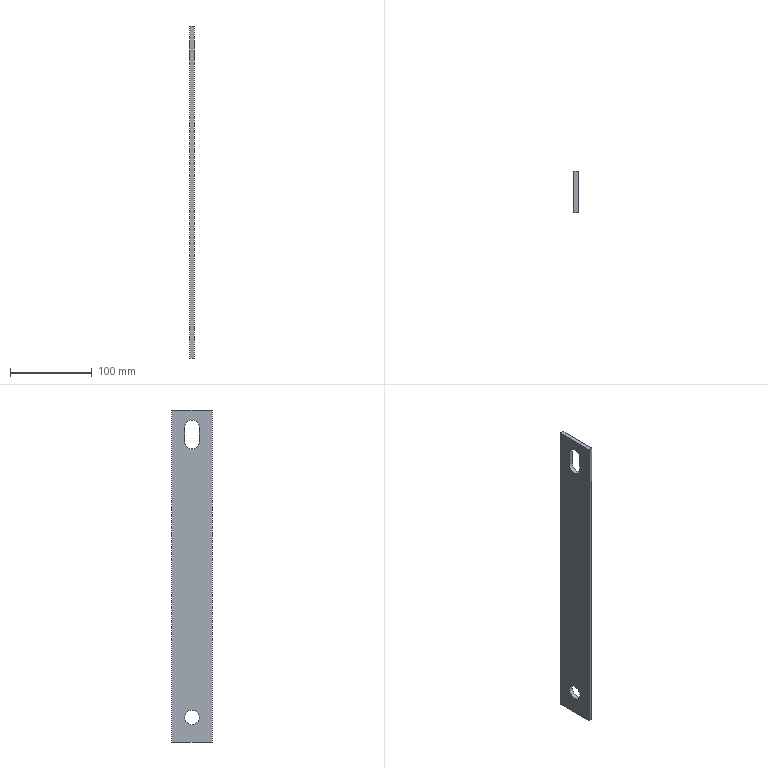Part | NX | features solid 2 | 1 solid | 11 faces | box 5 x 50 x 405 mm | volume 97175 mm3 | plane 8 | cylinder 3 | commonest cylinder face diameters 18 x3
STEP:
#1=CARTESIAN_POINT('',(1280.,720.,-185.));
#2=VERTEX_POINT('',#1);
#3=CARTESIAN_POINT('',(1280.,670.,-185.));
#4=VERTEX_POINT('',#3);
#5=CARTESIAN_POINT('',(1280.,695.,-185.));
#6=DIRECTION('',(0.,-1.,0.));
#7=VECTOR('',#6,1000.);
#8=LINE('',#5,#7);
#9=EDGE_CURVE('',#2,#4,#8,.T.);
#10=ORIENTED_EDGE('',*,*,#9,.F.);
#11=CARTESIAN_POINT('',(1285.,720.,-185.));
#12=VERTEX_POINT('',#11);
#13=CARTESIAN_POINT('',(1282.5,720.,-185.));
#14=DIRECTION('',(-1.,0.,0.));
#15=VECTOR('',#14,1000.);
#16=LINE('',#13,#15);
#17=EDGE_CURVE('',#12,#2,#16,.T.);
#18=ORIENTED_EDGE('',*,*,#17,.F.);
#19=CARTESIAN_POINT('',(1285.,670.,-185.));
#20=VERTEX_POINT('',#19);
#21=CARTESIAN_POINT('',(1285.,695.,-185.));
#22=DIRECTION('',(0.,1.,0.));
#23=VECTOR('',#22,1000.);
#24=LINE('',#21,#23);
#25=EDGE_CURVE('',#20,#12,#24,.T.);
#26=ORIENTED_EDGE('',*,*,#25,.F.);
#27=CARTESIAN_POINT('',(1282.5,670.,-185.));
#28=DIRECTION('',(1.,0.,0.));
#29=VECTOR('',#28,1000.);
#30=LINE('',#27,#29);
#31=EDGE_CURVE('',#4,#20,#30,.T.);
#32=ORIENTED_EDGE('',*,*,#31,.F.);
#33=EDGE_LOOP('',(#10,#18,#26,#32));
#34=FACE_BOUND('',#33,.T.);
#35=CARTESIAN_POINT('',(1272.5,695.,-185.));
#36=DIRECTION('',(0.,0.,-1.));
#37=DIRECTION('',(1.,0.,0.));
#38=AXIS2_PLACEMENT_3D('',#35,#36,#37);
#39=PLANE('',#38);
#40=ADVANCED_FACE('',(#34),#39,.T.);
#41=CARTESIAN_POINT('',(1285.,695.,-164.));
#42=VERTEX_POINT('',#41);
#43=CARTESIAN_POINT('',(1285.,695.,-155.));
#44=DIRECTION('',(-1.,0.,0.));
#45=DIRECTION('',(0.,0.,-1.));
#46=AXIS2_PLACEMENT_3D('',#43,#44,#45);
#47=CIRCLE('',#46,9.);
#48=EDGE_CURVE('',#42,#42,#47,.T.);
#49=ORIENTED_EDGE('',*,*,#48,.F.);
#50=EDGE_LOOP('',(#49));
#51=FACE_BOUND('',#50,.T.);
#52=CARTESIAN_POINT('',(1280.,695.,-146.));
#53=VERTEX_POINT('',#52);
#54=CARTESIAN_POINT('',(1280.,695.,-155.));
#55=DIRECTION('',(1.,0.,0.));
#56=DIRECTION('',(0.,0.,1.));
#57=AXIS2_PLACEMENT_3D('',#54,#55,#56);
#58=CIRCLE('',#57,9.);
#59=EDGE_CURVE('',#53,#53,#58,.T.);
#60=ORIENTED_EDGE('',*,*,#59,.F.);
#61=EDGE_LOOP('',(#60));
#62=FACE_BOUND('',#61,.T.);
#63=CARTESIAN_POINT('',(1280.,695.,-155.));
#64=DIRECTION('',(1.,0.,0.));
#65=DIRECTION('',(0.,0.,1.));
#66=AXIS2_PLACEMENT_3D('',#63,#64,#65);
#67=CYLINDRICAL_SURFACE('',#66,9.);
#68=ADVANCED_FACE('',(#51,#62),#67,.F.);
#69=ORIENTED_EDGE('',*,*,#59,.T.);
#70=EDGE_LOOP('',(#69));
#71=FACE_BOUND('',#70,.T.);
#72=CARTESIAN_POINT('',(1280.,670.,220.));
#73=VERTEX_POINT('',#72);
#74=CARTESIAN_POINT('',(1280.,670.,-215.));
#75=DIRECTION('',(0.,0.,1.));
#76=VECTOR('',#75,1000.);
#77=LINE('',#74,#76);
#78=EDGE_CURVE('',#4,#73,#77,.T.);
#79=ORIENTED_EDGE('',*,*,#78,.T.);
#80=CARTESIAN_POINT('',(1280.,720.,220.));
#81=VERTEX_POINT('',#80);
#82=CARTESIAN_POINT('',(1280.,695.,220.));
#83=DIRECTION('',(0.,1.,0.));
#84=VECTOR('',#83,1000.);
#85=LINE('',#82,#84);
#86=EDGE_CURVE('',#73,#81,#85,.T.);
#87=ORIENTED_EDGE('',*,*,#86,.T.);
#88=CARTESIAN_POINT('',(1280.,720.,-215.));
#89=DIRECTION('',(0.,0.,1.));
#90=VECTOR('',#89,1000.);
#91=LINE('',#88,#90);
#92=EDGE_CURVE('',#2,#81,#91,.T.);
#93=ORIENTED_EDGE('',*,*,#92,.F.);
#94=ORIENTED_EDGE('',*,*,#9,.T.);
#95=EDGE_LOOP('',(#79,#87,#93,#94));
#96=FACE_BOUND('',#95,.T.);
#97=CARTESIAN_POINT('',(1280.,704.,181.5));
#98=VERTEX_POINT('',#97);
#99=CARTESIAN_POINT('',(1280.,704.,198.5));
#100=VERTEX_POINT('',#99);
#101=CARTESIAN_POINT('',(1280.,704.,181.5));
#102=DIRECTION('',(0.,0.,1.));
#103=VECTOR('',#102,1000.);
#104=LINE('',#101,#103);
#105=EDGE_CURVE('',#98,#100,#104,.T.);
#106=ORIENTED_EDGE('',*,*,#105,.T.);
#107=CARTESIAN_POINT('',(1280.,686.,198.5));
#108=VERTEX_POINT('',#107);
#109=CARTESIAN_POINT('',(1280.,695.,198.5));
#110=DIRECTION('',(1.,0.,0.));
#111=DIRECTION('',(0.,0.,1.));
#112=AXIS2_PLACEMENT_3D('',#109,#110,#111);
#113=CIRCLE('',#112,9.);
#114=EDGE_CURVE('',#100,#108,#113,.T.);
#115=ORIENTED_EDGE('',*,*,#114,.T.);
#116=CARTESIAN_POINT('',(1280.,686.,181.5));
#117=VERTEX_POINT('',#116);
#118=CARTESIAN_POINT('',(1280.,686.,181.5));
#119=DIRECTION('',(0.,0.,1.));
#120=VECTOR('',#119,1000.);
#121=LINE('',#118,#120);
#122=EDGE_CURVE('',#117,#108,#121,.T.);
#123=ORIENTED_EDGE('',*,*,#122,.F.);
#124=CARTESIAN_POINT('',(1280.,695.,181.5));
#125=DIRECTION('',(1.,0.,0.));
#126=DIRECTION('',(0.,0.,1.));
#127=AXIS2_PLACEMENT_3D('',#124,#125,#126);
#128=CIRCLE('',#127,9.);
#129=EDGE_CURVE('',#117,#98,#128,.T.);
#130=ORIENTED_EDGE('',*,*,#129,.T.);
#131=EDGE_LOOP('',(#106,#115,#123,#130));
#132=FACE_BOUND('',#131,.T.);
#133=CARTESIAN_POINT('',(1280.,695.,-215.));
#134=DIRECTION('',(-1.,0.,0.));
#135=DIRECTION('',(0.,0.,-1.));
#136=AXIS2_PLACEMENT_3D('',#133,#134,#135);
#137=PLANE('',#136);
#138=ADVANCED_FACE('',(#71,#96,#132),#137,.T.);
#139=CARTESIAN_POINT('',(1285.,670.,220.));
#140=VERTEX_POINT('',#139);
#141=CARTESIAN_POINT('',(1285.,670.,-215.));
#142=DIRECTION('',(0.,0.,1.));
#143=VECTOR('',#142,1000.);
#144=LINE('',#141,#143);
#145=EDGE_CURVE('',#20,#140,#144,.T.);
#146=ORIENTED_EDGE('',*,*,#145,.T.);
#147=CARTESIAN_POINT('',(1282.5,670.,220.));
#148=DIRECTION('',(-1.,0.,0.));
#149=VECTOR('',#148,1000.);
#150=LINE('',#147,#149);
#151=EDGE_CURVE('',#140,#73,#150,.T.);
#152=ORIENTED_EDGE('',*,*,#151,.T.);
#153=ORIENTED_EDGE('',*,*,#78,.F.);
#154=ORIENTED_EDGE('',*,*,#31,.T.);
#155=EDGE_LOOP('',(#146,#152,#153,#154));
#156=FACE_BOUND('',#155,.T.);
#157=CARTESIAN_POINT('',(1282.5,670.,-215.));
#158=DIRECTION('',(0.,-1.,0.));
#159=DIRECTION('',(0.,0.,1.));
#160=AXIS2_PLACEMENT_3D('',#157,#158,#159);
#161=PLANE('',#160);
#162=ADVANCED_FACE('',(#156),#161,.T.);
#163=ORIENTED_EDGE('',*,*,#48,.T.);
#164=EDGE_LOOP('',(#163));
#165=FACE_BOUND('',#164,.T.);
#166=CARTESIAN_POINT('',(1285.,720.,220.));
#167=VERTEX_POINT('',#166);
#168=CARTESIAN_POINT('',(1285.,720.,-215.));
#169=DIRECTION('',(0.,0.,1.));
#170=VECTOR('',#169,1000.);
#171=LINE('',#168,#170);
#172=EDGE_CURVE('',#12,#167,#171,.T.);
#173=ORIENTED_EDGE('',*,*,#172,.T.);
#174=CARTESIAN_POINT('',(1285.,695.,220.));
#175=DIRECTION('',(0.,-1.,0.));
#176=VECTOR('',#175,1000.);
#177=LINE('',#174,#176);
#178=EDGE_CURVE('',#167,#140,#177,.T.);
#179=ORIENTED_EDGE('',*,*,#178,.T.);
#180=ORIENTED_EDGE('',*,*,#145,.F.);
#181=ORIENTED_EDGE('',*,*,#25,.T.);
#182=EDGE_LOOP('',(#173,#179,#180,#181));
#183=FACE_BOUND('',#182,.T.);
#184=CARTESIAN_POINT('',(1285.,704.,181.5));
#185=VERTEX_POINT('',#184);
#186=CARTESIAN_POINT('',(1285.,704.,198.5));
#187=VERTEX_POINT('',#186);
#188=CARTESIAN_POINT('',(1285.,704.,181.5));
#189=DIRECTION('',(0.,0.,1.));
#190=VECTOR('',#189,1000.);
#191=LINE('',#188,#190);
#192=EDGE_CURVE('',#185,#187,#191,.T.);
#193=ORIENTED_EDGE('',*,*,#192,.F.);
#194=CARTESIAN_POINT('',(1285.,686.,181.5));
#195=VERTEX_POINT('',#194);
#196=CARTESIAN_POINT('',(1285.,695.,181.5));
#197=DIRECTION('',(-1.,0.,0.));
#198=DIRECTION('',(0.,0.,-1.));
#199=AXIS2_PLACEMENT_3D('',#196,#197,#198);
#200=CIRCLE('',#199,9.);
#201=EDGE_CURVE('',#185,#195,#200,.T.);
#202=ORIENTED_EDGE('',*,*,#201,.T.);
#203=CARTESIAN_POINT('',(1285.,686.,198.5));
#204=VERTEX_POINT('',#203);
#205=CARTESIAN_POINT('',(1285.,686.,181.5));
#206=DIRECTION('',(0.,0.,1.));
#207=VECTOR('',#206,1000.);
#208=LINE('',#205,#207);
#209=EDGE_CURVE('',#195,#204,#208,.T.);
#210=ORIENTED_EDGE('',*,*,#209,.T.);
#211=CARTESIAN_POINT('',(1285.,695.,198.5));
#212=DIRECTION('',(-1.,0.,0.));
#213=DIRECTION('',(0.,0.,-1.));
#214=AXIS2_PLACEMENT_3D('',#211,#212,#213);
#215=CIRCLE('',#214,9.);
#216=EDGE_CURVE('',#204,#187,#215,.T.);
#217=ORIENTED_EDGE('',*,*,#216,.T.);
#218=EDGE_LOOP('',(#193,#202,#210,#217));
#219=FACE_BOUND('',#218,.T.);
#220=CARTESIAN_POINT('',(1285.,695.,-215.));
#221=DIRECTION('',(1.,0.,0.));
#222=DIRECTION('',(0.,0.,1.));
#223=AXIS2_PLACEMENT_3D('',#220,#221,#222);
#224=PLANE('',#223);
#225=ADVANCED_FACE('',(#165,#183,#219),#224,.T.);
#226=ORIENTED_EDGE('',*,*,#92,.T.);
#227=CARTESIAN_POINT('',(1282.5,720.,220.));
#228=DIRECTION('',(1.,0.,0.));
#229=VECTOR('',#228,1000.);
#230=LINE('',#227,#229);
#231=EDGE_CURVE('',#81,#167,#230,.T.);
#232=ORIENTED_EDGE('',*,*,#231,.T.);
#233=ORIENTED_EDGE('',*,*,#172,.F.);
#234=ORIENTED_EDGE('',*,*,#17,.T.);
#235=EDGE_LOOP('',(#226,#232,#233,#234));
#236=FACE_BOUND('',#235,.T.);
#237=CARTESIAN_POINT('',(1282.5,720.,-215.));
#238=DIRECTION('',(0.,1.,0.));
#239=DIRECTION('',(0.,0.,-1.));
#240=AXIS2_PLACEMENT_3D('',#237,#238,#239);
#241=PLANE('',#240);
#242=ADVANCED_FACE('',(#236),#241,.T.);
#243=CARTESIAN_POINT('',(1282.5,704.,198.5));
#244=DIRECTION('',(1.,0.,0.));
#245=VECTOR('',#244,1000.);
#246=LINE('',#243,#245);
#247=EDGE_CURVE('',#100,#187,#246,.T.);
#248=ORIENTED_EDGE('',*,*,#247,.T.);
#249=ORIENTED_EDGE('',*,*,#216,.F.);
#250=CARTESIAN_POINT('',(1282.5,686.,198.5));
#251=DIRECTION('',(-1.,0.,0.));
#252=VECTOR('',#251,1000.);
#253=LINE('',#250,#252);
#254=EDGE_CURVE('',#204,#108,#253,.T.);
#255=ORIENTED_EDGE('',*,*,#254,.T.);
#256=ORIENTED_EDGE('',*,*,#114,.F.);
#257=EDGE_LOOP('',(#248,#249,#255,#256));
#258=FACE_BOUND('',#257,.T.);
#259=CARTESIAN_POINT('',(1280.,695.,198.5));
#260=DIRECTION('',(1.,0.,0.));
#261=DIRECTION('',(0.,0.,1.));
#262=AXIS2_PLACEMENT_3D('',#259,#260,#261);
#263=CYLINDRICAL_SURFACE('',#262,9.);
#264=ADVANCED_FACE('',(#258),#263,.F.);
#265=ORIENTED_EDGE('',*,*,#231,.F.);
#266=ORIENTED_EDGE('',*,*,#86,.F.);
#267=ORIENTED_EDGE('',*,*,#151,.F.);
#268=ORIENTED_EDGE('',*,*,#178,.F.);
#269=EDGE_LOOP('',(#265,#266,#267,#268));
#270=FACE_BOUND('',#269,.T.);
#271=CARTESIAN_POINT('',(1272.5,695.,220.));
#272=DIRECTION('',(0.,0.,1.));
#273=DIRECTION('',(-1.,0.,0.));
#274=AXIS2_PLACEMENT_3D('',#271,#272,#273);
#275=PLANE('',#274);
#276=ADVANCED_FACE('',(#270),#275,.T.);
#277=ORIENTED_EDGE('',*,*,#201,.F.);
#278=CARTESIAN_POINT('',(1282.5,704.,181.5));
#279=DIRECTION('',(-1.,0.,0.));
#280=VECTOR('',#279,1000.);
#281=LINE('',#278,#280);
#282=EDGE_CURVE('',#185,#98,#281,.T.);
#283=ORIENTED_EDGE('',*,*,#282,.T.);
#284=ORIENTED_EDGE('',*,*,#129,.F.);
#285=CARTESIAN_POINT('',(1282.5,686.,181.5));
#286=DIRECTION('',(1.,0.,0.));
#287=VECTOR('',#286,1000.);
#288=LINE('',#285,#287);
#289=EDGE_CURVE('',#117,#195,#288,.T.);
#290=ORIENTED_EDGE('',*,*,#289,.T.);
#291=EDGE_LOOP('',(#277,#283,#284,#290));
#292=FACE_BOUND('',#291,.T.);
#293=CARTESIAN_POINT('',(1280.,695.,181.5));
#294=DIRECTION('',(1.,0.,0.));
#295=DIRECTION('',(0.,0.,1.));
#296=AXIS2_PLACEMENT_3D('',#293,#294,#295);
#297=CYLINDRICAL_SURFACE('',#296,9.);
#298=ADVANCED_FACE('',(#292),#297,.F.);
#299=ORIENTED_EDGE('',*,*,#209,.F.);
#300=ORIENTED_EDGE('',*,*,#289,.F.);
#301=ORIENTED_EDGE('',*,*,#122,.T.);
#302=ORIENTED_EDGE('',*,*,#254,.F.);
#303=EDGE_LOOP('',(#299,#300,#301,#302));
#304=FACE_BOUND('',#303,.T.);
#305=CARTESIAN_POINT('',(1282.5,686.,181.5));
#306=DIRECTION('',(0.,-1.,0.));
#307=DIRECTION('',(0.,0.,1.));
#308=AXIS2_PLACEMENT_3D('',#305,#306,#307);
#309=PLANE('',#308);
#310=ADVANCED_FACE('',(#304),#309,.F.);
#311=ORIENTED_EDGE('',*,*,#105,.F.);
#312=ORIENTED_EDGE('',*,*,#282,.F.);
#313=ORIENTED_EDGE('',*,*,#192,.T.);
#314=ORIENTED_EDGE('',*,*,#247,.F.);
#315=EDGE_LOOP('',(#311,#312,#313,#314));
#316=FACE_BOUND('',#315,.T.);
#317=CARTESIAN_POINT('',(1282.5,704.,181.5));
#318=DIRECTION('',(0.,1.,0.));
#319=DIRECTION('',(0.,0.,-1.));
#320=AXIS2_PLACEMENT_3D('',#317,#318,#319);
#321=PLANE('',#320);
#322=ADVANCED_FACE('',(#316),#321,.F.);
#323=CLOSED_SHELL('',(#40,#68,#138,#162,#225,#242,#264,#276,#298,#310,#322));
#324=MANIFOLD_SOLID_BREP('',#323);
#325=(LENGTH_UNIT()NAMED_UNIT(*)SI_UNIT(.MILLI.,.METRE.));
#326=UNCERTAINTY_MEASURE_WITH_UNIT(LENGTH_MEASURE(0.00001),#325,'','');
#327=(NAMED_UNIT(*)PLANE_ANGLE_UNIT()SI_UNIT($,.RADIAN.));
#328=(NAMED_UNIT(*)SI_UNIT($,.STERADIAN.)SOLID_ANGLE_UNIT());
#329=(GEOMETRIC_REPRESENTATION_CONTEXT(3)GLOBAL_UNCERTAINTY_ASSIGNED_CONTEXT((#326))GLOBAL_UNIT_ASSIGNED_CONTEXT((#325,#327,#328))REPRESENTATION_CONTEXT('',''));
#330=ADVANCED_BREP_SHAPE_REPRESENTATION('',(#324),#329);